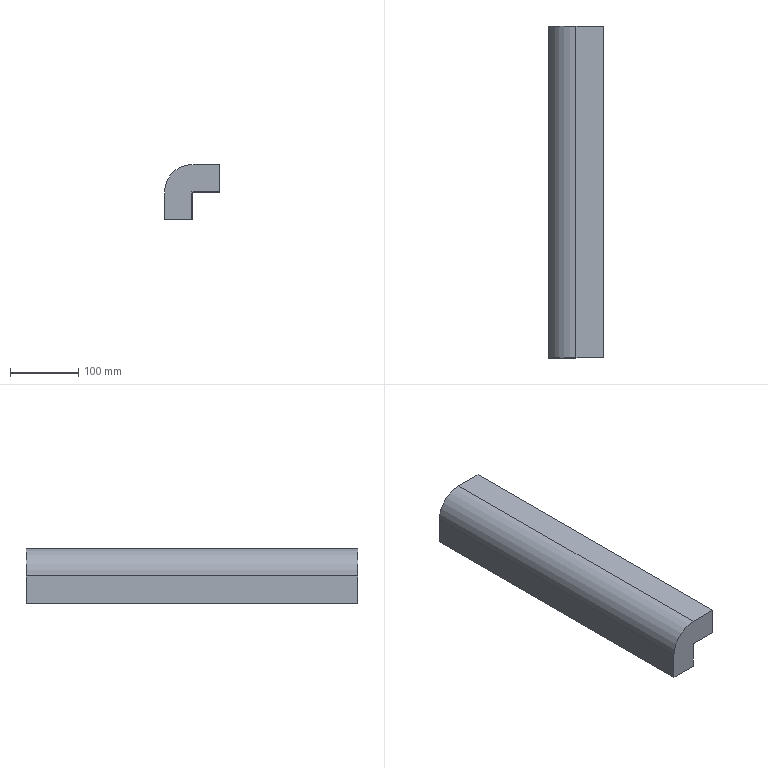Part | 1 solid | 18 faces | box 80 x 485 x 80 mm | volume 1821251 mm3 | plane 16 | cylinder 2 | commonest cylinder face diameters 76 x1 80 x1
STEP:
#1=CARTESIAN_POINT('',(-578.,440.,560.));
#2=VERTEX_POINT('',#1);
#3=CARTESIAN_POINT('',(-578.,925.,560.));
#4=VERTEX_POINT('',#3);
#5=CARTESIAN_POINT('',(-578.,1288.,560.));
#6=DIRECTION('',(0.,1.,0.));
#7=VECTOR('',#6,1000.);
#8=LINE('',#5,#7);
#9=EDGE_CURVE('',#2,#4,#8,.T.);
#10=ORIENTED_EDGE('',*,*,#9,.T.);
#11=CARTESIAN_POINT('',(-578.,925.,600.));
#12=VERTEX_POINT('',#11);
#13=CARTESIAN_POINT('',(-578.,925.,600.));
#14=DIRECTION('',(0.,0.,-1.));
#15=VECTOR('',#14,1000.);
#16=LINE('',#13,#15);
#17=EDGE_CURVE('',#12,#4,#16,.T.);
#18=ORIENTED_EDGE('',*,*,#17,.F.);
#19=CARTESIAN_POINT('',(-578.,440.,600.));
#20=VERTEX_POINT('',#19);
#21=CARTESIAN_POINT('',(-578.,461.5,600.));
#22=DIRECTION('',(0.,1.,0.));
#23=VECTOR('',#22,1000.);
#24=LINE('',#21,#23);
#25=EDGE_CURVE('',#20,#12,#24,.T.);
#26=ORIENTED_EDGE('',*,*,#25,.F.);
#27=CARTESIAN_POINT('',(-578.,440.,455.));
#28=DIRECTION('',(0.,0.,1.));
#29=VECTOR('',#28,1000.);
#30=LINE('',#27,#29);
#31=EDGE_CURVE('',#2,#20,#30,.T.);
#32=ORIENTED_EDGE('',*,*,#31,.F.);
#33=EDGE_LOOP('',(#10,#18,#26,#32));
#34=FACE_OUTER_BOUND('',#33,.T.);
#35=CARTESIAN_POINT('',(-578.,461.5,220.));
#36=DIRECTION('',(1.,0.,0.));
#37=DIRECTION('',(0.,0.,-1.));
#38=AXIS2_PLACEMENT_3D('',#35,#36,#37);
#39=PLANE('',#38);
#40=ADVANCED_FACE('',(#34),#39,.T.);
#41=CARTESIAN_POINT('',(-538.,925.,600.));
#42=VERTEX_POINT('',#41);
#43=CARTESIAN_POINT('',(-538.,440.,600.));
#44=VERTEX_POINT('',#43);
#45=CARTESIAN_POINT('',(-538.,461.5,600.));
#46=DIRECTION('',(0.,-1.,0.));
#47=VECTOR('',#46,1000.);
#48=LINE('',#45,#47);
#49=EDGE_CURVE('',#42,#44,#48,.T.);
#50=ORIENTED_EDGE('',*,*,#49,.F.);
#51=CARTESIAN_POINT('',(-538.,925.,640.));
#52=VERTEX_POINT('',#51);
#53=CARTESIAN_POINT('',(-538.,925.,565.1));
#54=DIRECTION('',(0.,0.,1.));
#55=VECTOR('',#54,1000.);
#56=LINE('',#53,#55);
#57=EDGE_CURVE('',#42,#52,#56,.T.);
#58=ORIENTED_EDGE('',*,*,#57,.T.);
#59=CARTESIAN_POINT('',(-538.,440.,640.));
#60=VERTEX_POINT('',#59);
#61=CARTESIAN_POINT('',(-538.,968.,640.));
#62=DIRECTION('',(0.,-1.,0.));
#63=VECTOR('',#62,1000.);
#64=LINE('',#61,#63);
#65=EDGE_CURVE('',#52,#60,#64,.T.);
#66=ORIENTED_EDGE('',*,*,#65,.T.);
#67=CARTESIAN_POINT('',(-538.,440.,455.));
#68=DIRECTION('',(0.,0.,1.));
#69=VECTOR('',#68,1000.);
#70=LINE('',#67,#69);
#71=EDGE_CURVE('',#44,#60,#70,.T.);
#72=ORIENTED_EDGE('',*,*,#71,.F.);
#73=EDGE_LOOP('',(#50,#58,#66,#72));
#74=FACE_OUTER_BOUND('',#73,.T.);
#75=CARTESIAN_POINT('',(-538.,968.,640.));
#76=DIRECTION('',(-1.,0.,0.));
#77=DIRECTION('',(0.,0.,1.));
#78=AXIS2_PLACEMENT_3D('',#75,#76,#77);
#79=PLANE('',#78);
#80=ADVANCED_FACE('',(#74),#79,.F.);
#81=CARTESIAN_POINT('',(-618.,440.,560.));
#82=VERTEX_POINT('',#81);
#83=CARTESIAN_POINT('',(-618.,925.,560.));
#84=VERTEX_POINT('',#83);
#85=CARTESIAN_POINT('',(-618.,968.,560.));
#86=DIRECTION('',(0.,1.,0.));
#87=VECTOR('',#86,1000.);
#88=LINE('',#85,#87);
#89=EDGE_CURVE('',#82,#84,#88,.T.);
#90=ORIENTED_EDGE('',*,*,#89,.T.);
#91=CARTESIAN_POINT('',(-538.,925.,560.));
#92=DIRECTION('',(1.,0.,0.));
#93=VECTOR('',#92,1000.);
#94=LINE('',#91,#93);
#95=EDGE_CURVE('',#84,#4,#94,.T.);
#96=ORIENTED_EDGE('',*,*,#95,.T.);
#97=ORIENTED_EDGE('',*,*,#9,.F.);
#98=CARTESIAN_POINT('',(-323.,440.,560.));
#99=DIRECTION('',(1.,0.,0.));
#100=VECTOR('',#99,1000.);
#101=LINE('',#98,#100);
#102=EDGE_CURVE('',#82,#2,#101,.T.);
#103=ORIENTED_EDGE('',*,*,#102,.F.);
#104=EDGE_LOOP('',(#90,#96,#97,#103));
#105=FACE_OUTER_BOUND('',#104,.T.);
#106=CARTESIAN_POINT('',(-578.,1288.,560.));
#107=DIRECTION('',(0.,0.,1.));
#108=DIRECTION('',(1.,0.,0.));
#109=AXIS2_PLACEMENT_3D('',#106,#107,#108);
#110=PLANE('',#109);
#111=ADVANCED_FACE('',(#105),#110,.F.);
#112=CARTESIAN_POINT('',(-618.,440.,600.));
#113=VERTEX_POINT('',#112);
#114=CARTESIAN_POINT('',(-578.,440.,640.));
#115=VERTEX_POINT('',#114);
#116=CARTESIAN_POINT('',(-578.,440.,600.));
#117=DIRECTION('',(0.,1.,0.));
#118=DIRECTION('',(-1.,0.,0.));
#119=AXIS2_PLACEMENT_3D('',#116,#117,#118);
#120=CIRCLE('',#119,40.);
#121=EDGE_CURVE('',#113,#115,#120,.T.);
#122=ORIENTED_EDGE('',*,*,#121,.F.);
#123=CARTESIAN_POINT('',(-618.,440.,800.));
#124=DIRECTION('',(0.,0.,-1.));
#125=VECTOR('',#124,1000.);
#126=LINE('',#123,#125);
#127=EDGE_CURVE('',#113,#82,#126,.T.);
#128=ORIENTED_EDGE('',*,*,#127,.T.);
#129=ORIENTED_EDGE('',*,*,#102,.T.);
#130=ORIENTED_EDGE('',*,*,#31,.T.);
#131=CARTESIAN_POINT('',(-323.,440.,600.));
#132=DIRECTION('',(1.,0.,0.));
#133=VECTOR('',#132,1000.);
#134=LINE('',#131,#133);
#135=EDGE_CURVE('',#20,#44,#134,.T.);
#136=ORIENTED_EDGE('',*,*,#135,.T.);
#137=ORIENTED_EDGE('',*,*,#71,.T.);
#138=CARTESIAN_POINT('',(-538.,440.,640.));
#139=DIRECTION('',(-1.,0.,0.));
#140=VECTOR('',#139,1000.);
#141=LINE('',#138,#140);
#142=EDGE_CURVE('',#60,#115,#141,.T.);
#143=ORIENTED_EDGE('',*,*,#142,.T.);
#144=EDGE_LOOP('',(#122,#128,#129,#130,#136,#137,#143));
#145=FACE_OUTER_BOUND('',#144,.T.);
#146=CARTESIAN_POINT('',(-323.,440.,455.));
#147=DIRECTION('',(0.,-1.,0.));
#148=DIRECTION('',(-1.,0.,0.));
#149=AXIS2_PLACEMENT_3D('',#146,#147,#148);
#150=PLANE('',#149);
#151=ADVANCED_FACE('',(#145),#150,.T.);
#152=CARTESIAN_POINT('',(-618.,925.,600.));
#153=VERTEX_POINT('',#152);
#154=CARTESIAN_POINT('',(-618.,1288.,600.));
#155=DIRECTION('',(0.,-1.,0.));
#156=VECTOR('',#155,1000.);
#157=LINE('',#154,#156);
#158=EDGE_CURVE('',#153,#113,#157,.T.);
#159=ORIENTED_EDGE('',*,*,#158,.F.);
#160=CARTESIAN_POINT('',(-618.,925.,565.1));
#161=DIRECTION('',(0.,0.,1.));
#162=VECTOR('',#161,1000.);
#163=LINE('',#160,#162);
#164=EDGE_CURVE('',#84,#153,#163,.T.);
#165=ORIENTED_EDGE('',*,*,#164,.F.);
#166=ORIENTED_EDGE('',*,*,#89,.F.);
#167=ORIENTED_EDGE('',*,*,#127,.F.);
#168=EDGE_LOOP('',(#159,#165,#166,#167));
#169=FACE_OUTER_BOUND('',#168,.T.);
#170=CARTESIAN_POINT('',(-618.,968.,800.));
#171=DIRECTION('',(1.,0.,0.));
#172=DIRECTION('',(0.,0.,-1.));
#173=AXIS2_PLACEMENT_3D('',#170,#171,#172);
#174=PLANE('',#173);
#175=ADVANCED_FACE('',(#169),#174,.F.);
#176=ORIENTED_EDGE('',*,*,#65,.F.);
#177=CARTESIAN_POINT('',(-578.,925.,640.));
#178=VERTEX_POINT('',#177);
#179=CARTESIAN_POINT('',(-538.,925.,640.));
#180=DIRECTION('',(-1.,0.,0.));
#181=VECTOR('',#180,1000.);
#182=LINE('',#179,#181);
#183=EDGE_CURVE('',#52,#178,#182,.T.);
#184=ORIENTED_EDGE('',*,*,#183,.T.);
#185=CARTESIAN_POINT('',(-578.,1288.,640.));
#186=DIRECTION('',(0.,1.,0.));
#187=VECTOR('',#186,1000.);
#188=LINE('',#185,#187);
#189=EDGE_CURVE('',#115,#178,#188,.T.);
#190=ORIENTED_EDGE('',*,*,#189,.F.);
#191=ORIENTED_EDGE('',*,*,#142,.F.);
#192=EDGE_LOOP('',(#176,#184,#190,#191));
#193=FACE_OUTER_BOUND('',#192,.T.);
#194=CARTESIAN_POINT('',(-538.,968.,640.));
#195=DIRECTION('',(0.,0.,-1.));
#196=DIRECTION('',(-1.,0.,0.));
#197=AXIS2_PLACEMENT_3D('',#194,#195,#196);
#198=PLANE('',#197);
#199=ADVANCED_FACE('',(#193),#198,.F.);
#200=ORIENTED_EDGE('',*,*,#189,.T.);
#201=CARTESIAN_POINT('',(-578.,925.,600.));
#202=DIRECTION('',(0.,1.,0.));
#203=DIRECTION('',(0.,0.,1.));
#204=AXIS2_PLACEMENT_3D('',#201,#202,#203);
#205=CIRCLE('',#204,40.);
#206=EDGE_CURVE('',#153,#178,#205,.T.);
#207=ORIENTED_EDGE('',*,*,#206,.F.);
#208=ORIENTED_EDGE('',*,*,#158,.T.);
#209=ORIENTED_EDGE('',*,*,#121,.T.);
#210=EDGE_LOOP('',(#200,#207,#208,#209));
#211=FACE_OUTER_BOUND('',#210,.T.);
#212=CARTESIAN_POINT('',(-578.,1288.,600.));
#213=DIRECTION('',(0.,-1.,0.));
#214=DIRECTION('',(-1.,0.,0.));
#215=AXIS2_PLACEMENT_3D('',#212,#213,#214);
#216=CYLINDRICAL_SURFACE('',#215,40.);
#217=ADVANCED_FACE('',(#211),#216,.T.);
#218=ORIENTED_EDGE('',*,*,#25,.T.);
#219=CARTESIAN_POINT('',(-538.,925.,600.));
#220=DIRECTION('',(-1.,0.,0.));
#221=VECTOR('',#220,1000.);
#222=LINE('',#219,#221);
#223=EDGE_CURVE('',#42,#12,#222,.T.);
#224=ORIENTED_EDGE('',*,*,#223,.F.);
#225=ORIENTED_EDGE('',*,*,#49,.T.);
#226=ORIENTED_EDGE('',*,*,#135,.F.);
#227=EDGE_LOOP('',(#218,#224,#225,#226));
#228=FACE_OUTER_BOUND('',#227,.T.);
#229=CARTESIAN_POINT('',(242.,461.5,600.));
#230=DIRECTION('',(0.,0.,-1.));
#231=DIRECTION('',(-1.,0.,0.));
#232=AXIS2_PLACEMENT_3D('',#229,#230,#231);
#233=PLANE('',#232);
#234=ADVANCED_FACE('',(#228),#233,.T.);
#235=ORIENTED_EDGE('',*,*,#164,.T.);
#236=ORIENTED_EDGE('',*,*,#206,.T.);
#237=ORIENTED_EDGE('',*,*,#183,.F.);
#238=ORIENTED_EDGE('',*,*,#57,.F.);
#239=ORIENTED_EDGE('',*,*,#223,.T.);
#240=ORIENTED_EDGE('',*,*,#17,.T.);
#241=ORIENTED_EDGE('',*,*,#95,.F.);
#242=EDGE_LOOP('',(#235,#236,#237,#238,#239,#240,#241));
#243=FACE_OUTER_BOUND('',#242,.T.);
#244=CARTESIAN_POINT('',(-538.,925.,565.1));
#245=DIRECTION('',(0.,1.,0.));
#246=DIRECTION('',(0.,0.,1.));
#247=AXIS2_PLACEMENT_3D('',#244,#245,#246);
#248=PLANE('',#247);
#249=ADVANCED_FACE('',(#243),#248,.T.);
#250=CLOSED_SHELL('',(#40,#80,#111,#151,#175,#199,#217,#234,#249));
#251=CARTESIAN_POINT('',(-540.,442.,638.));
#252=VERTEX_POINT('',#251);
#253=CARTESIAN_POINT('',(-578.,442.,638.));
#254=VERTEX_POINT('',#253);
#255=CARTESIAN_POINT('',(-540.,442.,638.));
#256=DIRECTION('',(-1.,0.,0.));
#257=VECTOR('',#256,1000.);
#258=LINE('',#255,#257);
#259=EDGE_CURVE('',#252,#254,#258,.T.);
#260=ORIENTED_EDGE('',*,*,#259,.F.);
#261=CARTESIAN_POINT('',(-540.,442.,602.));
#262=VERTEX_POINT('',#261);
#263=CARTESIAN_POINT('',(-540.,442.,638.));
#264=DIRECTION('',(0.,0.,-1.));
#265=VECTOR('',#264,1000.);
#266=LINE('',#263,#265);
#267=EDGE_CURVE('',#252,#262,#266,.T.);
#268=ORIENTED_EDGE('',*,*,#267,.T.);
#269=CARTESIAN_POINT('',(-580.,442.,602.));
#270=VERTEX_POINT('',#269);
#271=CARTESIAN_POINT('',(-580.,442.,602.));
#272=DIRECTION('',(1.,0.,0.));
#273=VECTOR('',#272,1000.);
#274=LINE('',#271,#273);
#275=EDGE_CURVE('',#270,#262,#274,.T.);
#276=ORIENTED_EDGE('',*,*,#275,.F.);
#277=CARTESIAN_POINT('',(-580.,442.,562.));
#278=VERTEX_POINT('',#277);
#279=CARTESIAN_POINT('',(-580.,442.,636.9));
#280=DIRECTION('',(0.,0.,-1.));
#281=VECTOR('',#280,1000.);
#282=LINE('',#279,#281);
#283=EDGE_CURVE('',#270,#278,#282,.T.);
#284=ORIENTED_EDGE('',*,*,#283,.T.);
#285=CARTESIAN_POINT('',(-616.,442.,562.));
#286=VERTEX_POINT('',#285);
#287=CARTESIAN_POINT('',(-616.,442.,562.));
#288=DIRECTION('',(1.,0.,0.));
#289=VECTOR('',#288,1000.);
#290=LINE('',#287,#289);
#291=EDGE_CURVE('',#286,#278,#290,.T.);
#292=ORIENTED_EDGE('',*,*,#291,.F.);
#293=CARTESIAN_POINT('',(-616.,442.,600.));
#294=VERTEX_POINT('',#293);
#295=CARTESIAN_POINT('',(-616.,442.,636.9));
#296=DIRECTION('',(0.,0.,-1.));
#297=VECTOR('',#296,1000.);
#298=LINE('',#295,#297);
#299=EDGE_CURVE('',#294,#286,#298,.T.);
#300=ORIENTED_EDGE('',*,*,#299,.F.);
#301=CARTESIAN_POINT('',(-578.,442.,600.));
#302=DIRECTION('',(0.,1.,0.));
#303=DIRECTION('',(1.,0.,0.));
#304=AXIS2_PLACEMENT_3D('',#301,#302,#303);
#305=CIRCLE('',#304,38.);
#306=EDGE_CURVE('',#294,#254,#305,.T.);
#307=ORIENTED_EDGE('',*,*,#306,.T.);
#308=EDGE_LOOP('',(#260,#268,#276,#284,#292,#300,#307));
#309=FACE_OUTER_BOUND('',#308,.T.);
#310=CARTESIAN_POINT('',(-580.,442.,562.));
#311=DIRECTION('',(0.,1.,0.));
#312=DIRECTION('',(1.,0.,0.));
#313=AXIS2_PLACEMENT_3D('',#310,#311,#312);
#314=PLANE('',#313);
#315=ADVANCED_FACE('',(#309),#314,.T.);
#316=CARTESIAN_POINT('',(-540.,530.,638.));
#317=VERTEX_POINT('',#316);
#318=CARTESIAN_POINT('',(-578.,530.,638.));
#319=VERTEX_POINT('',#318);
#320=CARTESIAN_POINT('',(-540.,530.,638.));
#321=DIRECTION('',(-1.,0.,0.));
#322=VECTOR('',#321,1000.);
#323=LINE('',#320,#322);
#324=EDGE_CURVE('',#317,#319,#323,.T.);
#325=ORIENTED_EDGE('',*,*,#324,.T.);
#326=CARTESIAN_POINT('',(-616.,530.,600.));
#327=VERTEX_POINT('',#326);
#328=CARTESIAN_POINT('',(-578.,530.,600.));
#329=DIRECTION('',(0.,-1.,0.));
#330=DIRECTION('',(0.,0.,-1.));
#331=AXIS2_PLACEMENT_3D('',#328,#329,#330);
#332=CIRCLE('',#331,38.);
#333=EDGE_CURVE('',#319,#327,#332,.T.);
#334=ORIENTED_EDGE('',*,*,#333,.T.);
#335=CARTESIAN_POINT('',(-616.,530.,562.));
#336=VERTEX_POINT('',#335);
#337=CARTESIAN_POINT('',(-616.,530.,638.));
#338=DIRECTION('',(0.,0.,-1.));
#339=VECTOR('',#338,1000.);
#340=LINE('',#337,#339);
#341=EDGE_CURVE('',#327,#336,#340,.T.);
#342=ORIENTED_EDGE('',*,*,#341,.T.);
#343=CARTESIAN_POINT('',(-580.,530.,562.));
#344=VERTEX_POINT('',#343);
#345=CARTESIAN_POINT('',(-616.,530.,562.));
#346=DIRECTION('',(1.,0.,0.));
#347=VECTOR('',#346,1000.);
#348=LINE('',#345,#347);
#349=EDGE_CURVE('',#336,#344,#348,.T.);
#350=ORIENTED_EDGE('',*,*,#349,.T.);
#351=CARTESIAN_POINT('',(-580.,530.,602.));
#352=VERTEX_POINT('',#351);
#353=CARTESIAN_POINT('',(-580.,530.,562.));
#354=DIRECTION('',(0.,0.,1.));
#355=VECTOR('',#354,1000.);
#356=LINE('',#353,#355);
#357=EDGE_CURVE('',#344,#352,#356,.T.);
#358=ORIENTED_EDGE('',*,*,#357,.T.);
#359=CARTESIAN_POINT('',(-540.,530.,602.));
#360=VERTEX_POINT('',#359);
#361=CARTESIAN_POINT('',(-580.,530.,602.));
#362=DIRECTION('',(1.,0.,0.));
#363=VECTOR('',#362,1000.);
#364=LINE('',#361,#363);
#365=EDGE_CURVE('',#352,#360,#364,.T.);
#366=ORIENTED_EDGE('',*,*,#365,.T.);
#367=CARTESIAN_POINT('',(-540.,530.,602.));
#368=DIRECTION('',(0.,0.,1.));
#369=VECTOR('',#368,1000.);
#370=LINE('',#367,#369);
#371=EDGE_CURVE('',#360,#317,#370,.T.);
#372=ORIENTED_EDGE('',*,*,#371,.T.);
#373=EDGE_LOOP('',(#325,#334,#342,#350,#358,#366,#372));
#374=FACE_OUTER_BOUND('',#373,.T.);
#375=CARTESIAN_POINT('',(0.,530.,0.));
#376=DIRECTION('',(0.,-1.,0.));
#377=DIRECTION('',(0.,0.,-1.));
#378=AXIS2_PLACEMENT_3D('',#375,#376,#377);
#379=PLANE('',#378);
#380=ADVANCED_FACE('',(#374),#379,.T.);
#381=ORIENTED_EDGE('',*,*,#306,.F.);
#382=CARTESIAN_POINT('',(-616.,4.,600.));
#383=DIRECTION('',(0.,-1.,0.));
#384=VECTOR('',#383,1000.);
#385=LINE('',#382,#384);
#386=EDGE_CURVE('',#327,#294,#385,.T.);
#387=ORIENTED_EDGE('',*,*,#386,.F.);
#388=ORIENTED_EDGE('',*,*,#333,.F.);
#389=CARTESIAN_POINT('',(-578.,2.,638.));
#390=DIRECTION('',(0.,1.,0.));
#391=VECTOR('',#390,1000.);
#392=LINE('',#389,#391);
#393=EDGE_CURVE('',#254,#319,#392,.T.);
#394=ORIENTED_EDGE('',*,*,#393,.F.);
#395=EDGE_LOOP('',(#381,#387,#388,#394));
#396=FACE_OUTER_BOUND('',#395,.T.);
#397=CARTESIAN_POINT('',(-578.,2.,600.));
#398=DIRECTION('',(0.,1.,0.));
#399=DIRECTION('',(0.,0.,1.));
#400=AXIS2_PLACEMENT_3D('',#397,#398,#399);
#401=CYLINDRICAL_SURFACE('',#400,38.);
#402=ADVANCED_FACE('',(#396),#401,.F.);
#403=ORIENTED_EDGE('',*,*,#341,.F.);
#404=ORIENTED_EDGE('',*,*,#386,.T.);
#405=ORIENTED_EDGE('',*,*,#299,.T.);
#406=CARTESIAN_POINT('',(-616.,530.,562.));
#407=DIRECTION('',(0.,-1.,0.));
#408=VECTOR('',#407,1000.);
#409=LINE('',#406,#408);
#410=EDGE_CURVE('',#336,#286,#409,.T.);
#411=ORIENTED_EDGE('',*,*,#410,.F.);
#412=EDGE_LOOP('',(#403,#404,#405,#411));
#413=FACE_OUTER_BOUND('',#412,.T.);
#414=CARTESIAN_POINT('',(-616.,4.,636.9));
#415=DIRECTION('',(-1.,0.,0.));
#416=DIRECTION('',(0.,0.,1.));
#417=AXIS2_PLACEMENT_3D('',#414,#415,#416);
#418=PLANE('',#417);
#419=ADVANCED_FACE('',(#413),#418,.F.);
#420=ORIENTED_EDGE('',*,*,#410,.T.);
#421=ORIENTED_EDGE('',*,*,#291,.T.);
#422=CARTESIAN_POINT('',(-580.,4.,562.));
#423=DIRECTION('',(0.,1.,0.));
#424=VECTOR('',#423,1000.);
#425=LINE('',#422,#424);
#426=EDGE_CURVE('',#278,#344,#425,.T.);
#427=ORIENTED_EDGE('',*,*,#426,.T.);
#428=ORIENTED_EDGE('',*,*,#349,.F.);
#429=EDGE_LOOP('',(#420,#421,#427,#428));
#430=FACE_OUTER_BOUND('',#429,.T.);
#431=CARTESIAN_POINT('',(0.,2.,562.));
#432=DIRECTION('',(0.,0.,1.));
#433=DIRECTION('',(1.,0.,0.));
#434=AXIS2_PLACEMENT_3D('',#431,#432,#433);
#435=PLANE('',#434);
#436=ADVANCED_FACE('',(#430),#435,.T.);
#437=CARTESIAN_POINT('',(-580.,516.1,602.));
#438=DIRECTION('',(0.,-1.,0.));
#439=VECTOR('',#438,1000.);
#440=LINE('',#437,#439);
#441=EDGE_CURVE('',#352,#270,#440,.T.);
#442=ORIENTED_EDGE('',*,*,#441,.F.);
#443=ORIENTED_EDGE('',*,*,#357,.F.);
#444=ORIENTED_EDGE('',*,*,#426,.F.);
#445=ORIENTED_EDGE('',*,*,#283,.F.);
#446=EDGE_LOOP('',(#442,#443,#444,#445));
#447=FACE_OUTER_BOUND('',#446,.T.);
#448=CARTESIAN_POINT('',(-580.,516.1,636.9));
#449=DIRECTION('',(1.,0.,0.));
#450=DIRECTION('',(0.,0.,-1.));
#451=AXIS2_PLACEMENT_3D('',#448,#449,#450);
#452=PLANE('',#451);
#453=ADVANCED_FACE('',(#447),#452,.F.);
#454=CARTESIAN_POINT('',(-540.,4.,602.));
#455=DIRECTION('',(0.,1.,0.));
#456=VECTOR('',#455,1000.);
#457=LINE('',#454,#456);
#458=EDGE_CURVE('',#262,#360,#457,.T.);
#459=ORIENTED_EDGE('',*,*,#458,.T.);
#460=ORIENTED_EDGE('',*,*,#365,.F.);
#461=ORIENTED_EDGE('',*,*,#441,.T.);
#462=ORIENTED_EDGE('',*,*,#275,.T.);
#463=EDGE_LOOP('',(#459,#460,#461,#462));
#464=FACE_OUTER_BOUND('',#463,.T.);
#465=CARTESIAN_POINT('',(0.,2.,602.));
#466=DIRECTION('',(0.,0.,1.));
#467=DIRECTION('',(1.,0.,0.));
#468=AXIS2_PLACEMENT_3D('',#465,#466,#467);
#469=PLANE('',#468);
#470=ADVANCED_FACE('',(#464),#469,.T.);
#471=ORIENTED_EDGE('',*,*,#267,.F.);
#472=CARTESIAN_POINT('',(-540.,507.9,638.));
#473=DIRECTION('',(0.,-1.,0.));
#474=VECTOR('',#473,1000.);
#475=LINE('',#472,#474);
#476=EDGE_CURVE('',#317,#252,#475,.T.);
#477=ORIENTED_EDGE('',*,*,#476,.F.);
#478=ORIENTED_EDGE('',*,*,#371,.F.);
#479=ORIENTED_EDGE('',*,*,#458,.F.);
#480=EDGE_LOOP('',(#471,#477,#478,#479));
#481=FACE_OUTER_BOUND('',#480,.T.);
#482=CARTESIAN_POINT('',(-540.,17.9,638.));
#483=DIRECTION('',(1.,0.,0.));
#484=DIRECTION('',(0.,0.,-1.));
#485=AXIS2_PLACEMENT_3D('',#482,#483,#484);
#486=PLANE('',#485);
#487=ADVANCED_FACE('',(#481),#486,.F.);
#488=ORIENTED_EDGE('',*,*,#476,.T.);
#489=ORIENTED_EDGE('',*,*,#259,.T.);
#490=ORIENTED_EDGE('',*,*,#393,.T.);
#491=ORIENTED_EDGE('',*,*,#324,.F.);
#492=EDGE_LOOP('',(#488,#489,#490,#491));
#493=FACE_OUTER_BOUND('',#492,.T.);
#494=CARTESIAN_POINT('',(0.,2.,638.));
#495=DIRECTION('',(0.,0.,-1.));
#496=DIRECTION('',(-1.,0.,0.));
#497=AXIS2_PLACEMENT_3D('',#494,#495,#496);
#498=PLANE('',#497);
#499=ADVANCED_FACE('',(#493),#498,.T.);
#500=CLOSED_SHELL('',(#315,#380,#402,#419,#436,#453,#470,#487,#499));
#501=ORIENTED_CLOSED_SHELL('',*,#500,.F.);
#502=BREP_WITH_VOIDS('',#250,(#501));
#503=CARTESIAN_POINT('',(0.,0.,0.));
#504=DIRECTION('',(0.,0.,1.));
#505=DIRECTION('',(1.,0.,0.));
#506=AXIS2_PLACEMENT_3D('',#503,#504,#505);
#507=(LENGTH_UNIT()NAMED_UNIT(*)SI_UNIT(.MILLI.,.METRE.));
#508=UNCERTAINTY_MEASURE_WITH_UNIT(LENGTH_MEASURE(0.00001),#507,'','');
#509=(NAMED_UNIT(*)PLANE_ANGLE_UNIT()SI_UNIT($,.RADIAN.));
#510=(NAMED_UNIT(*)SI_UNIT($,.STERADIAN.)SOLID_ANGLE_UNIT());
#511=(GEOMETRIC_REPRESENTATION_CONTEXT(3)GLOBAL_UNCERTAINTY_ASSIGNED_CONTEXT((#508))GLOBAL_UNIT_ASSIGNED_CONTEXT((#507,#509,#510))REPRESENTATION_CONTEXT('',''));
#512=ADVANCED_BREP_SHAPE_REPRESENTATION('',(#502,#506),#511);